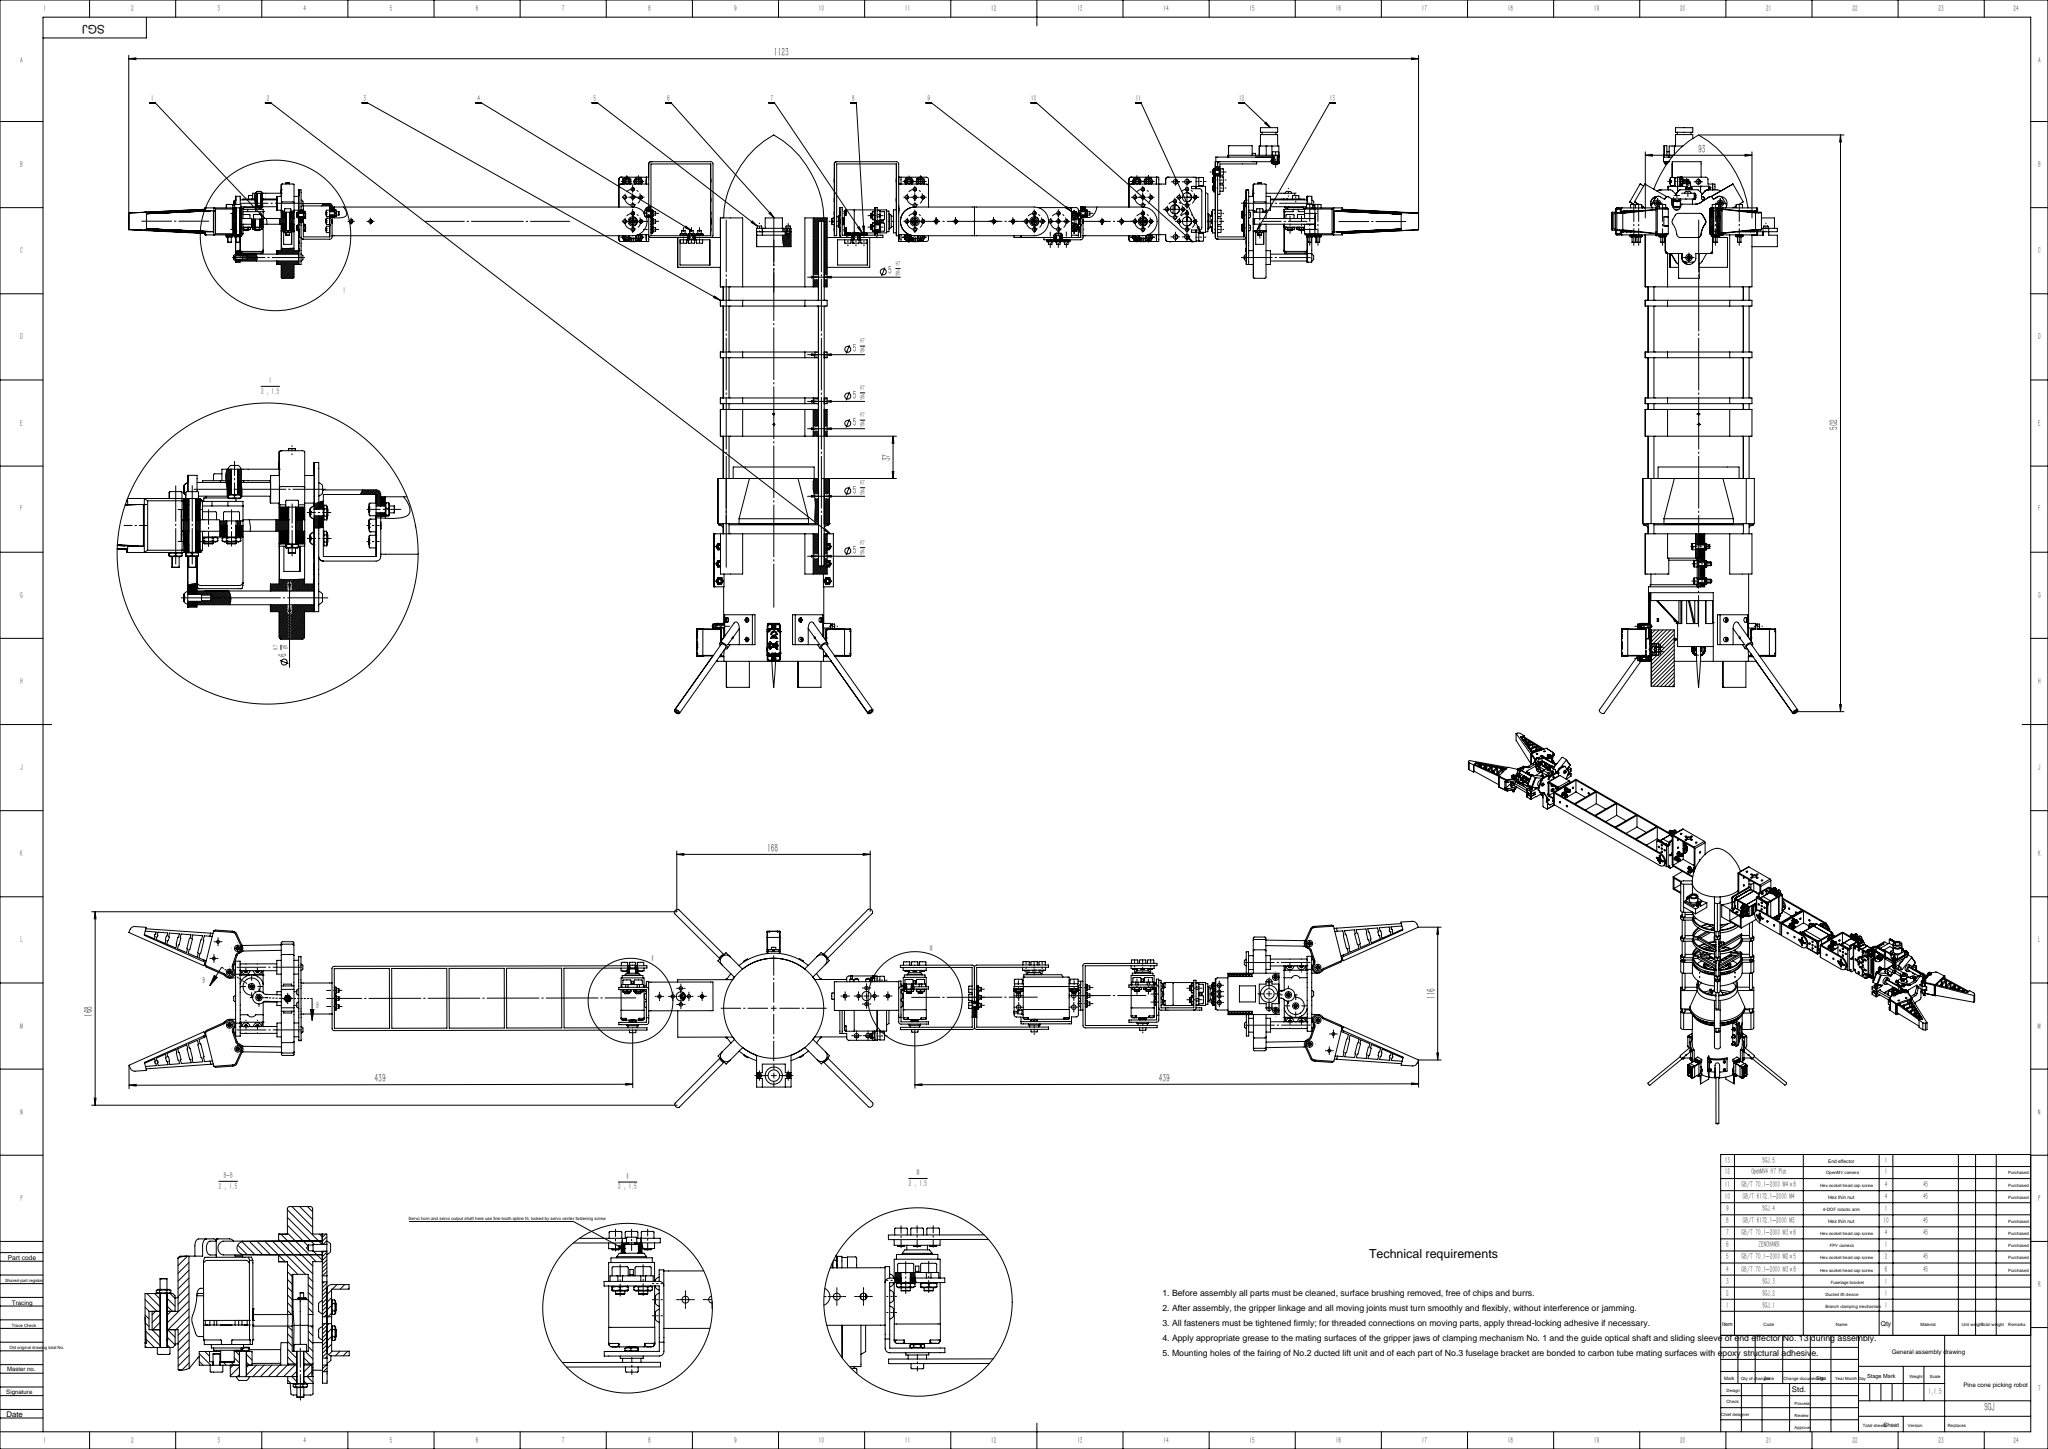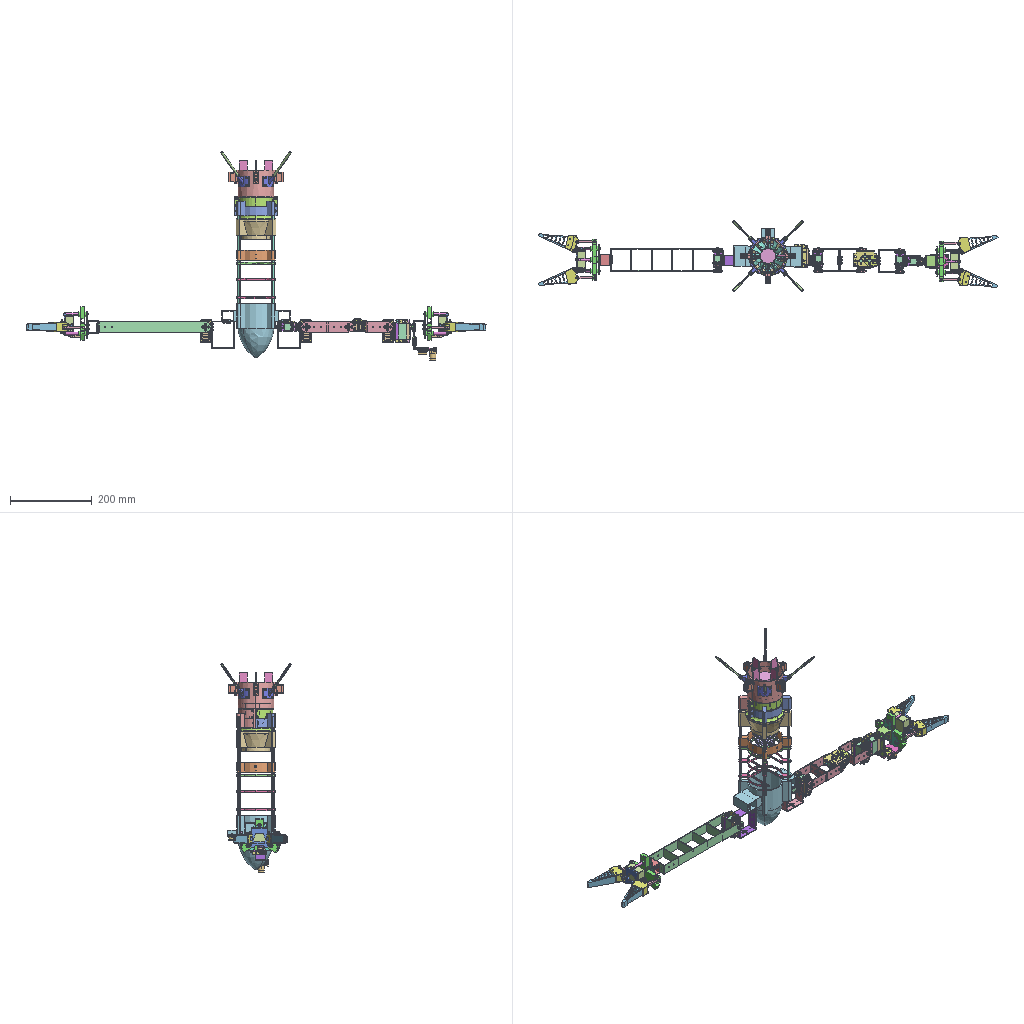Assembly | SolidWorks | 47 different items | 106 placed | box 1123 x 173 x 510 mm
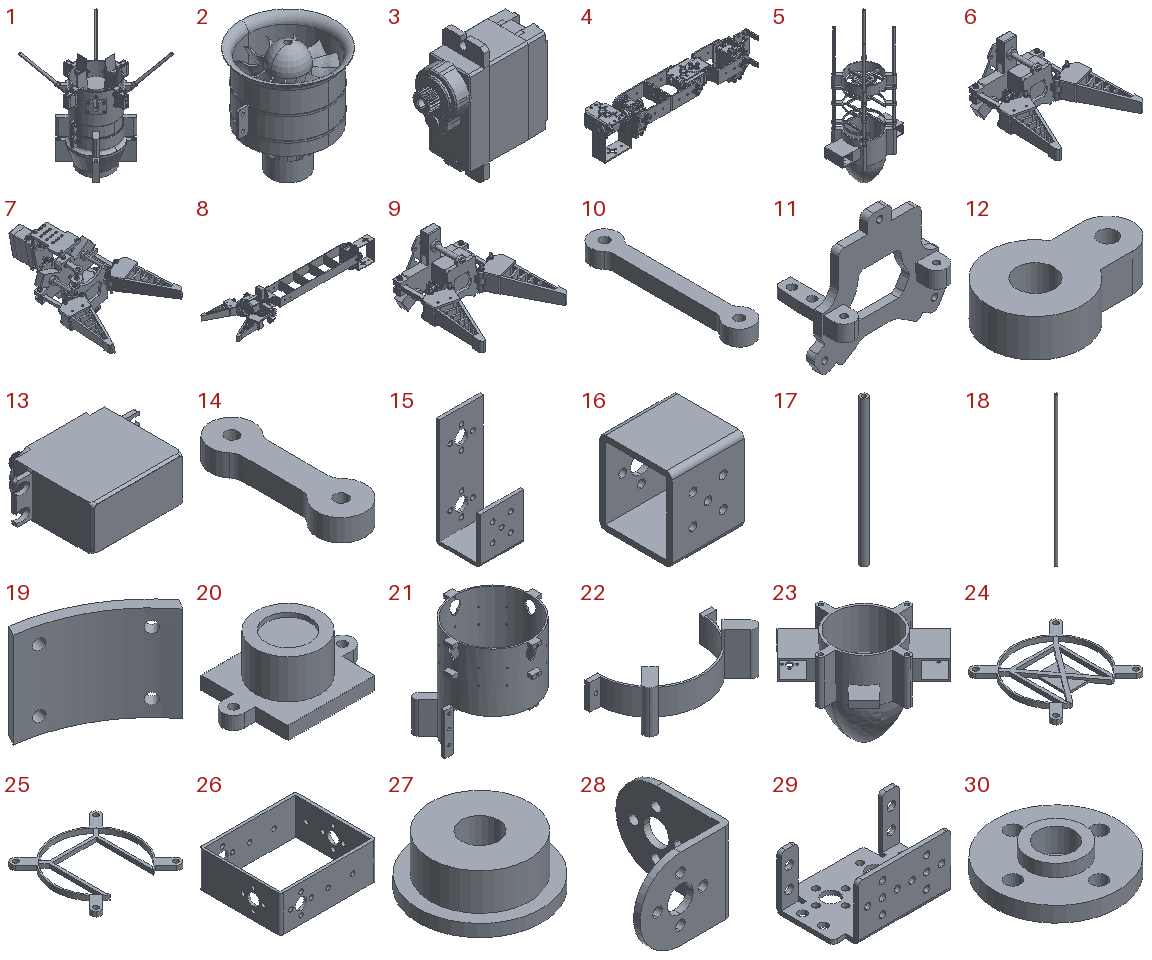Parts list (item | name | quantity | parent item | size | volume | features):
1 | (subassembly) | x1 | - | - | 344611 mm3 | features ReferencePattern 9, CompositeCurve 7, LocalCirPattern 2
2 | (subassembly) | x1 | in 1 | 103 x 96 x 111.255 mm | 142445 mm3 | features CompositeCurve 2
3 | (subassembly) | x4 | in 1 | 29 x 11.559 x 32.1 mm | 6256 mm3 | -
4 | (subassembly) | x1 | - | - | 161976 mm3 | features CompositeCurve 8
5 | (subassembly) | x1 | - | 167.293 x 115.141 x 375.279 mm | 493659 mm3 | features ReferencePattern 3, CompositeCurve 1, LocalCirPattern 1
6 | (subassembly) | x1 | in 7 | 125.947 x 151.548 x 83 mm | 142512 mm3 | -
7 | (subassembly) | x1 | - | 126.41 x 222.148 x 108.699 mm | 180398 mm3 | features CompositeCurve 2
8 | (subassembly) | x1 | - | - | 229160 mm3 | features CompositeCurve 1
9 | (subassembly) | x1 | in 8 | 125.947 x 151.548 x 83 mm | 142512 mm3 | -
10 | - | x4 | in 6, 9 | 9 x 52.5 x 5 mm | 1409 mm3 | features BaseBody 1
11 | - | x2 | in 6, 9 | 65.292 x 34.3 x 57.348 mm | 10403 mm3 | features ICE 10, Fillet 6, HoleWzd 2, Extrusion 1, MirrorPattern 1
12 | - | x2 | in 6, 9 | 23 x 15 x 6 mm | 1241 mm3 | features BaseBody 1, Cut 1
13 | - | x2 | in 6, 9 | 56 x 45.5 x 20 mm | 31577 mm3 | features Cut 2, BaseBody 1
14 | - | x2 | in 6, 9 | 11 x 35.5 x 5 mm | 1255 mm3 | features BaseBody 1
15 | - | x1 | in 7 | 27 x 27 x 67.5 mm | 6022 mm3 | features ICE 5, Extrusion 1, Fillet 1
16 | - | x1 | in 8 | 27 x 27 x 31 mm | 5512 mm3 | features ICE 4, Fillet 2, Extrusion 1
17 | - | x4 | in 1 | 5 x 5 x 100 mm | 1470 mm3 | features Extrusion 1, ICE 1
18 | - | x4 | in 5 | 5 x 5 x 300 mm | 4418 mm3 | features Extrusion 1
19 | - | x4 | in 1 | 31.064 x 30.415 x 29.867 mm | 3679 mm3 | features ICE 5, CirPattern 1, Extrusion 1
20 | - | x1 | - | 30 x 20 x 12 mm | 2827 mm3 | features ICE 4, Extrusion 1, Fillet 1, MirrorPattern 1
21 | - | x1 | in 1 | 104 x 99.2 x 110.99 mm | 51523 mm3 | features ICE 12, CirPattern 4, Fillet 2, HoleWzd 2, Extrusion 1
22 | - | x1 | in 1 | 104 x 47.686 x 35 mm | 18349 mm3 | features ICE 8, Fillet 2, CirPattern 1, Extrusion 1
23 | - | x1 | in 5 | 153.584 x 153.584 x 132.279 mm | 420410 mm3 | features ICE 10, MirrorPattern 2, CirPattern 1, Extrusion 1, Fillet 1, HoleWzd 1, Revolution 1
24 | - | x1 | in 5 | 92.873 x 92.873 x 5 mm | 10601 mm3 | features ICE 6, CirPattern 1, Extrusion 1, Fillet 1
25 | - | x2 | in 5 | 92.873 x 92.873 x 5 mm | 7282 mm3 | features ICE 4, CirPattern 1, Extrusion 1, Fillet 1
26 | - | x1 | in 8 | 66 x 56 x 25 mm | 10390 mm3 | features ICE 5, Fillet 2, Extrusion 1, MirrorPattern 1
27 | - | x5 | in 4, 8 | 10 x 10 x 4 mm | 201.062 mm3 | features ICE 2, Extrusion 1
28 | - | x2 | in 4, 7 | 28.5 x 34 x 25 mm | 2421 mm3 | features Fillet 3, ICE 3, Extrusion 1
29 | - | x6 | in 4, 8 | 56 x 37.49 x 26 mm | 5821 mm3 | features ICE 8, LPattern 2, Extrusion 1, Fillet 1, MirrorPattern 1
30 | - | x6 | in 4, 7, 8 | 20 x 20 x 4.5 mm | 753.693 mm3 | features ICE 4, Extrusion 1, HoleWzd 1
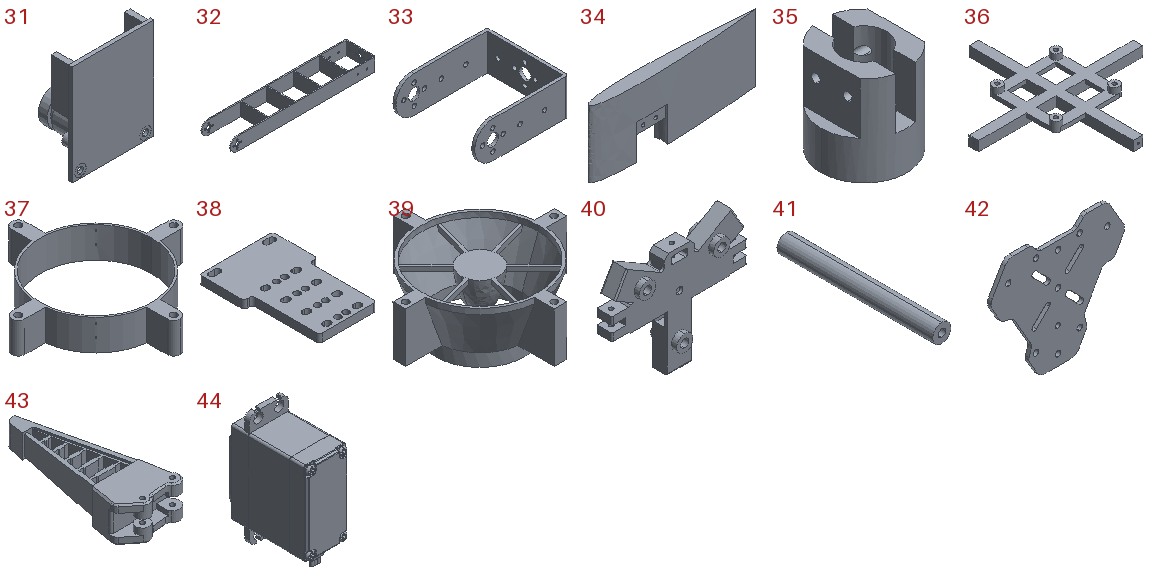31 | - | x1 | - | 36 x 25.6 x 44.5 mm | 8664 mm3 | features BaseBody 1
32 | - | x1 | in 8 | 274.25 x 56 x 25 mm | 39558 mm3 | features ICE 5, Fillet 3, Extrusion 1
33 | - | x4 | in 4 | 64.5 x 56 x 25 mm | 8183 mm3 | features Fillet 3, ICE 3, Extrusion 1, MirrorPattern 1
34 | - | x4 | in 1 | 50 x 4.001 x 20 mm | 2418 mm3 | features ICE 3, CurveInFile 1, Extrusion 1
35 | - | x4 | in 1 | 10 x 10 x 10.5 mm | 483.8 mm3 | features ICE 6, Extrusion 1
36 | - | x1 | in 5 | 84.2 x 84.2 x 8 mm | 5113 mm3 | features ICE 9, Extrusion 1
37 | - | x1 | in 5 | 127.2 x 127.2 x 23.3 mm | 25300 mm3 | features ICE 3, CirPattern 2, Extrusion 1, Fillet 1
38 | - | x1 | in 7 | 36 x 55 x 4 mm | 6185 mm3 | features ICE 2, Extrusion 1, Fillet 1
39 | - | x1 | in 1 | 127.2 x 127.2 x 49.3 mm | 72395 mm3 | features ICE 8, CirPattern 2, Revolution 2, Shell 1
40 | - | x2 | in 6, 9 | 99 x 19 x 82.044 mm | 35178 mm3 | features ICE 7, Revolution 6, Fillet 5, HoleWzd 5, MirrorPattern 5, Chamfer 1, Extrusion 1
41 | - | x6 | in 6, 9 | 6 x 51 x 6 mm | 1381 mm3 | features HoleWzd 2, BaseBody 1
42 | - | x2 | in 6, 9 | 73.405 x 2 x 64.91 mm | 5563 mm3 | features BaseBody 1
43 | - | x4 | in 6, 9 | 40.322 x 99.83 x 23.5 mm | 23198 mm3 | features BaseBody 2, Cut 1
44 | - | x6 | in 4, 7, 8 | 20.1 x 44.6 x 55.6 mm | 21079 mm3 | features ICE 27, Fillet 16, Chamfer 2, CombineBodies 2, Extrusion 1, HoleWzd 1, LPattern 1, Revolution 1
45 | hex thin nuts-grades ab-chamfered gb | x1 | - | - | - | -
46 | hexagon socket button head screws gb | x1 | - | - | - | -
47 | hexagon socket head cap screws gb | x1 | - | - | - | -
Mates (type | each side: item.copy, entity, surface, feature):
In the top assembly
Coincident | 38.1 face plane Boss-Extrude1 | 31.1 face plane Input1 | 3 times
Concentric | 21.1 face cylinder Cut-Extrude5 | 18.1 face cylinder Boss-Extrude1
Coincident | 21.1 face plane Cut-Extrude5 | 18.1 face plane Boss-Extrude1
Lock | 21.1 select_type:0 | 18.1 select_type:0
Concentric | 39.1 face cylinder Cut-Extrude3 | 37.1 face cylinder CirPattern1
Coincident | 23.1 face plane Boss-Extrude5 | 20.1 face plane Boss-Extrude1
Concentric | 20.1 face cylinder Cut-Extrude1 | 23.1 edge
Concentric | 23.1 edge | 20.1 edge
Coincident | 23.1 face plane Boss-Extrude3 | 29.1 face plane Boss-Extrude1
Concentric | 23.1 face cylinder Cut-Extrude5 | 29.1 face cylinder Cut-Extrude4 | 2 times
Coincident | 29.2 face plane Boss-Extrude3 | 44.1 face plane Boss-Extrude3
Concentric | 29.2 face cylinder Cut-Extrude6 | 44.1 face cylinder Cut-Extrude4 | 2 times
Coincident | 23.1 face plane Mirror2 | 26.1 face plane Boss-Extrude2
Concentric | 23.1 face cylinder Cut-Extrude7 | 26.1 face cylinder Cut-Extrude5 | 2 times
In subassembly 8
Coincident | 26.2 face plane Boss-Extrude1 | 29.3 face plane Boss-Extrude1
Concentric | 26.2 face cylinder Mirror1 | 29.3 face cylinder Cut-Extrude4 | 2 times
Coincident | 29.3 face plane LinPattern1 | 44.2 face plane Boss-Extrude3
Concentric | 29.3 face cylinder Mirror2 | 44.2 face cylinder Cut-Extrude4 | 2 times
Coincident | 29.3 face plane Boss-Extrude1 | 27.1 face plane Boss-Extrude1
Concentric | 29.3 face cylinder Cut-Extrude5 | 27.1 face cylinder Cut-Extrude2
Lock | 29.3 select_type:0 | 27.1 select_type:0
Parallel | 29.3 face plane Boss-Extrude1 | 32.1 face plane Boss-Extrude1
Coincident | 44.2 face plane Boss-Extrude9 | 30.1 face plane Cut-Extrude3
Concentric | 44.2 face cylinder Boss-Extrude9 | 30.1 face cylinder Cut-Extrude3
Coincident | 30.1 face plane Boss-Extrude1 | 32.1 face plane Cut-Extrude1
Concentric | 30.1 face cylinder Cut-Extrude4 | 32.1 face cylinder Cut-Extrude3
Concentric | 32.1 face cylinder Cut-Extrude3 | 30.1 edge
Coincident | 32.1 face plane Boss-Extrude1 | 16.1 face plane Boss-Extrude1
Concentric | 32.1 face cylinder Cut-Extrude2 | 16.1 face cylinder Cut-Extrude2 | 2 times
Coincident | 16.1 face plane Boss-Extrude1 | 42.1 face plane Input1
Concentric | 16.1 face cylinder Cut-Extrude3 | 42.1 face cylinder Input1 | 2 times
In subassembly 9
Lock | 41.1 select_type:0 | 42.2 select_type:0
Concentric | 13.1 face cylinder Input1 | 12.1 face cylinder Input1 | 2 times
DistanceDim | 13.1 face plane Input1 | 12.1 face plane Input1
Concentric | 14.1 face cylinder Input1 | 12.1 face cylinder Input1
Coincident | 14.1 face plane Input1 | 12.1 face plane Input1
Coincident | 13.1 face plane Input1 | 11.1 face plane Boss-Extrude2
DistanceDim | 11.1 face plane Boss-Extrude1 | 13.1 face plane Input1
Coincident | 13.1 face plane Input1 | 11.1 face plane Boss-Extrude1
Lock | 41.1 select_type:0 | 11.1 select_type:0
Lock | 41.2 select_type:0 | 11.1 select_type:0
Lock | 41.3 select_type:0 | 11.1 select_type:0
Concentric | 41.3 face cylinder Input1 | 40.1 face cylinder Ø6.0 (6) Dia Hole1
Concentric | 41.1 face cylinder Input1 | 40.1 face cylinder Ø6.0 (6) Dia Hole1
Concentric | 14.1 face cylinder Input1 | 40.1 face cylinder Ø3.0 (3) Dia Hole7
Concentric | 40.1 face cylinder Mirror7 | 10.1 face cylinder Input1
Width | 10.1 face plane Input1 | 10.1 face plane Input1 | 40.1 face plane Mirror4 | 40.1 face plane Mirror4
Concentric | 10.1 face cylinder Input1 | 43.1 face cylinder Input1
Width | 10.1 face plane Input1 | 10.1 face plane Input1 | 43.1 face plane Input1 | 43.1 face plane Input1
Concentric | 11.1 face cylinder Cut-Extrude6 | 43.1 face cylinder Input1
Concentric | 40.1 face cylinder Cut-Extrude14 | 10.2 face cylinder Input1
Width | 10.2 face plane Input1 | 10.2 face plane Input1 | 40.1 face plane Cut-Extrude12 | 40.1 face plane Cut-Extrude12
Concentric | 43.2 face cylinder Input1 | 10.2 face cylinder Input1
Width | 10.2 face plane Input1 | 10.2 face plane Input1 | 43.2 face plane Input1 | 43.2 face plane Input1
Concentric | 11.1 face cylinder Mirror1 | 43.2 face cylinder Input1
LimitDistanceDim | 40.1 face plane Revolve5 | 42.2 face plane Input1
In subassembly 4
Concentric | 29.3 face cylinder Cut-Extrude6 | 44.2 face cylinder Cut-Extrude4
Concentric | 29.3 face cylinder Mirror2 | 44.2 face cylinder Cut-Extrude4
Coincident | 29.3 face plane LinPattern1 | 44.2 face plane Boss-Extrude3
Coincident | 29.3 face plane Boss-Extrude1 | 27.1 face plane Boss-Extrude1
Concentric | 29.3 face cylinder Cut-Extrude5 | 27.1 face cylinder Cut-Extrude2
Lock | 29.3 select_type:0 | 27.1 select_type:0
Parallel | 29.3 face plane Cut-Extrude1 | 33.1 face plane Boss-Extrude1
Coincident | 44.2 face plane Boss-Extrude9 | 30.1 face plane Cut-Extrude3
Concentric | 44.2 face cylinder Boss-Extrude9 | 30.1 face cylinder Cut-Extrude3
Concentric | 33.1 face cylinder Cut-Extrude3 | 30.1 edge
Coincident | 30.1 face plane Boss-Extrude1 | 33.1 face plane Cut-Extrude1
Concentric | 33.1 face cylinder Mirror1 | 30.1 edge
Concentric | 29.4 face cylinder Cut-Extrude4 | 33.1 face cylinder Mirror1 | 2 times
Coincident | 29.4 face plane Boss-Extrude1 | 33.1 face plane Boss-Extrude1
Concentric | 29.4 face cylinder Mirror2 | 44.3 face cylinder Cut-Extrude4 | 2 times
Coincident | 29.4 face plane LinPattern1 | 44.3 face plane Boss-Extrude3
Coincident | 29.4 face plane Boss-Extrude1 | 27.2 face plane Boss-Extrude1
Concentric | 29.4 face cylinder Cut-Extrude5 | 27.2 face cylinder Cut-Extrude2
Lock | 29.4 select_type:0 | 27.2 select_type:0
Parallel | 29.4 face plane Boss-Extrude1 | 33.2 face plane Boss-Extrude1
Coincident | 44.3 face plane Boss-Extrude9 | 30.2 face plane Cut-Extrude3
Concentric | 44.3 face cylinder Boss-Extrude9 | 30.2 face cylinder Cut-Extrude3
Concentric | 33.2 face cylinder Mirror1 | 30.2 edge | 2 times
Coincident | 30.2 face plane Boss-Extrude1 | 33.2 face plane Cut-Extrude1
Concentric | 33.2 face cylinder Cut-Extrude2 | 33.3 face cylinder Cut-Extrude2 | 2 times
Coincident | 33.2 face plane Boss-Extrude1 | 33.3 face plane Boss-Extrude1
Concentric | 33.3 face cylinder Cut-Extrude3 | 30.3 edge | 2 times
Coincident | 33.3 face plane Cut-Extrude1 | 30.3 face plane Boss-Extrude1
Parallel | 33.3 face plane Boss-Extrude1 | 29.5 face plane Boss-Extrude2
Concentric | 44.4 face cylinder Cut-Extrude4 | 29.5 face cylinder Cut-Extrude6 | 2 times
Coincident | 44.4 face plane Boss-Extrude3 | 29.5 face plane Boss-Extrude3
Concentric | 44.4 face cylinder Boss-Extrude9 | 30.3 face cylinder Cut-Extrude3
Coincident | 44.4 face plane Boss-Extrude9 | 30.3 face plane Cut-Extrude3
Coincident | 29.5 face plane Boss-Extrude1 | 27.3 face plane Boss-Extrude1
Concentric | 29.5 face cylinder Cut-Extrude5 | 27.3 face cylinder Cut-Extrude2
Coincident | 29.5 face plane Boss-Extrude1 | 28.1 face plane Cut-Extrude3
Concentric | 29.5 face cylinder Cut-Extrude4 | 28.1 face cylinder Cut-Extrude4 | 2 times
Lock | 29.5 select_type:0 | 27.3 select_type:0
Concentric | 28.1 face cylinder Cut-Extrude5 | 33.4 face cylinder Cut-Extrude2 | 2 times
Coincident | 28.1 face plane Boss-Extrude1 | 33.4 face plane Boss-Extrude1
Coincident | 33.4 face plane Cut-Extrude1 | 30.4 face plane Boss-Extrude1
Concentric | 33.4 face cylinder Mirror1 | 30.4 edge | 2 times
Parallel | 33.4 face plane Boss-Extrude1 | 29.6 face plane Boss-Extrude1
Concentric | 44.5 face cylinder Cut-Extrude4 | 29.6 face cylinder Cut-Extrude6 | 2 times
Coincident | 44.5 face plane Boss-Extrude3 | 29.6 face plane Boss-Extrude3
Coincident | 44.5 face plane Boss-Extrude9 | 30.4 face plane Cut-Extrude3
Concentric | 30.4 face cylinder Cut-Extrude3 | 44.5 face cylinder Boss-Extrude9
Coincident | 29.7 face plane Boss-Extrude1 | 29.6 face plane Boss-Extrude1
Concentric | 29.7 face cylinder Cut-Extrude5 | 29.6 face cylinder Cut-Extrude4 | 2 times
Coincident | 27.4 face plane Boss-Extrude1 | 29.6 face plane Boss-Extrude1
Concentric | 27.4 face cylinder Cut-Extrude2 | 29.6 face cylinder Cut-Extrude5
Lock | 27.4 select_type:0 | 29.6 select_type:0
In subassembly 1
Coincident | 21.2 face plane Cut-Extrude2 | 22.1 face plane Cut-Extrude1
Concentric | 21.2 face cylinder Cut-Extrude4 | 22.1 face cylinder Cut-Extrude2
Coincident | 21.2 face plane Boss-Extrude1 | 22.1 face plane Boss-Extrude1
Concentric | 21.2 face cylinder CirPattern3 | 19.1 face cylinder Cut-Extrude1
Concentric | 21.2 face cylinder CirPattern3 | 19.1 face cylinder CirPattern1
Parallel | 21.2 face plane CirPattern4 | 35.1 face plane Cut-Extrude3
Parallel | 21.2 face plane Boss-Extrude5 | 35.2 face plane Cut-Extrude3
Parallel | 21.2 face plane CirPattern4 | 35.3 face plane Cut-Extrude3
Parallel | 21.2 face plane CirPattern4 | 35.4 face plane Cut-Extrude3
Concentric | 19.1 face cylinder Boss-Extrude2 | 17.1 face cylinder Boss-Extrude1
Lock | 19.1 select_type:0 | 17.1 select_type:0
Concentric | 34.1 face cylinder Cut-Extrude2 | 35.1 face cylinder Cut-Extrude6 | 2 times
Coincident | 34.1 face plane Boss-Extrude2 | 35.1 face plane Cut-Extrude4
Concentric | 34.2 face cylinder Cut-Extrude2 | 35.4 face cylinder Cut-Extrude6 | 2 times
Coincident | 34.2 face plane Boss-Extrude2 | 35.4 face plane Cut-Extrude4
Concentric | 35.2 face cylinder Cut-Extrude6 | 34.3 face cylinder Cut-Extrude2 | 2 times
Coincident | 35.2 face plane Cut-Extrude4 | 34.3 face plane Boss-Extrude2
Concentric | 34.4 face cylinder Cut-Extrude2 | 35.3 face cylinder Cut-Extrude6 | 2 times
Coincident | 34.4 face plane Boss-Extrude2 | 35.3 face plane Cut-Extrude4
In subassembly 5
Concentric | 18.2 face cylinder Boss-Extrude1 | 25.1 face cylinder Cut-Extrude3
Concentric | 18.2 face cylinder Boss-Extrude1 | 24.1 face cylinder Cut-Extrude3
Concentric | 18.2 face cylinder Boss-Extrude1 | 25.2 face cylinder Cut-Extrude3
Coincident | 18.2 face cylinder Boss-Extrude1 | 37.2 edge
Concentric | 18.2 face cylinder Boss-Extrude1 | 23.2 face cylinder CirPattern1
Coincident | 18.2 face plane Boss-Extrude1 | 23.2 face plane CirPattern1
Concentric | 37.2 face cylinder CirPattern2 | 36.1 face cylinder Cut-Extrude6
Concentric | 37.2 face cylinder CirPattern2 | 36.1 face cylinder Cut-Extrude5
DistanceDim | 24.1 face plane Boss-Extrude1 | 37.2 face plane Boss-Extrude1
DistanceDim | 25.1 face plane Boss-Extrude1 | 24.1 face plane Boss-Extrude1
Concentric | 24.1 face cylinder CirPattern1 | 18.3 face cylinder Boss-Extrude1
DistanceDim | 25.2 face plane Boss-Extrude1 | 25.1 face plane Boss-Extrude1
DistanceDim | 25.2 face plane Boss-Extrude1 | 23.2 face plane Boss-Extrude1
Concentric | 25.2 face cylinder CirPattern1 | 18.3 face cylinder Boss-Extrude1
Concentric | 25.1 face cylinder CirPattern1 | 18.3 face cylinder Boss-Extrude1
Concentric | 23.2 face cylinder CirPattern1 | 18.3 face cylinder Boss-Extrude1
In subassembly 7
Coincident | 15.1 face plane Boss-Extrude1 | 42.3 face plane Input1
Concentric | 15.1 face cylinder Cut-Extrude3 | 42.3 face cylinder Input1 | 2 times
Coincident | 15.1 face plane Cut-Extrude1 | 28.1 face plane Boss-Extrude1
Concentric | 15.1 face cylinder Cut-Extrude4 | 28.1 face cylinder Cut-Extrude5 | 2 times
Coincident | 38.2 face plane Boss-Extrude1 | 28.1 face plane Boss-Extrude1
Concentric | 28.1 face cylinder Cut-Extrude4 | 38.2 face cylinder Cut-Extrude1
Concentric | 38.2 face cylinder Cut-Extrude1 | 28.1 face cylinder Cut-Extrude4
Concentric | 44.2 face cylinder Boss-Extrude9 | 30.1 face cylinder Cut-Extrude3
Coincident | 44.2 face plane Boss-Extrude9 | 30.1 face plane Cut-Extrude3
Coincident | 15.1 face plane Boss-Extrude1 | 30.1 face plane Boss-Extrude1
Concentric | 15.1 face cylinder Cut-Extrude2 | 30.1 edge | 2 times
Parallel | 15.1 face plane Boss-Extrude1 | 44.2 face plane Boss-Extrude4
In subassembly 6
Lock | 41.1 select_type:0 | 42.2 select_type:0
Concentric | 13.1 face cylinder Input1 | 12.1 face cylinder Input1
DistanceDim | 13.1 face plane Input1 | 12.1 face plane Input1
Concentric | 14.1 face cylinder Input1 | 12.1 face cylinder Input1
Coincident | 14.1 face plane Input1 | 12.1 face plane Input1
Coincident | 13.1 face plane Input1 | 11.1 face plane Boss-Extrude2
DistanceDim | 11.1 face plane Boss-Extrude1 | 13.1 face plane Input1
Coincident | 13.1 face plane Input1 | 11.1 face plane Boss-Extrude1
Lock | 41.1 select_type:0 | 11.1 select_type:0
Lock | 41.2 select_type:0 | 11.1 select_type:0
Lock | 41.3 select_type:0 | 11.1 select_type:0
Concentric | 41.3 face cylinder Input1 | 40.1 face cylinder Ø6.0 (6) Dia Hole1
Concentric | 41.1 face cylinder Input1 | 40.1 face cylinder Ø6.0 (6) Dia Hole1
Concentric | 14.1 face cylinder Input1 | 40.1 face cylinder Ø3.0 (3) Dia Hole7
Concentric | 40.1 face cylinder Mirror7 | 10.1 face cylinder Input1
Width | 10.1 face plane Input1 | 10.1 face plane Input1 | 40.1 face plane Mirror4 | 40.1 face plane Mirror4
Concentric | 10.1 face cylinder Input1 | 43.1 face cylinder Cut-Extrude1
Width | 10.1 face plane Input1 | 10.1 face plane Input1 | 43.1 face plane Input1 | 43.1 face plane Input1
Concentric | 11.1 face cylinder Cut-Extrude6 | 43.1 face cylinder Cut-Extrude1
Concentric | 40.1 face cylinder Cut-Extrude14 | 10.2 face cylinder Input1
Width | 10.2 face plane Input1 | 10.2 face plane Input1 | 40.1 face plane Cut-Extrude12 | 40.1 face plane Cut-Extrude12
Concentric | 10.2 face cylinder Input1 | 43.2 face cylinder Cut-Extrude1
Width | 10.2 face plane Input1 | 10.2 face plane Input1 | 43.2 face plane Input1 | 43.2 face plane Input1
Concentric | 11.1 face cylinder Mirror1 | 43.2 face cylinder Cut-Extrude1
LimitDistanceDim | 40.1 face plane Revolve5 | 42.2 face plane Input1